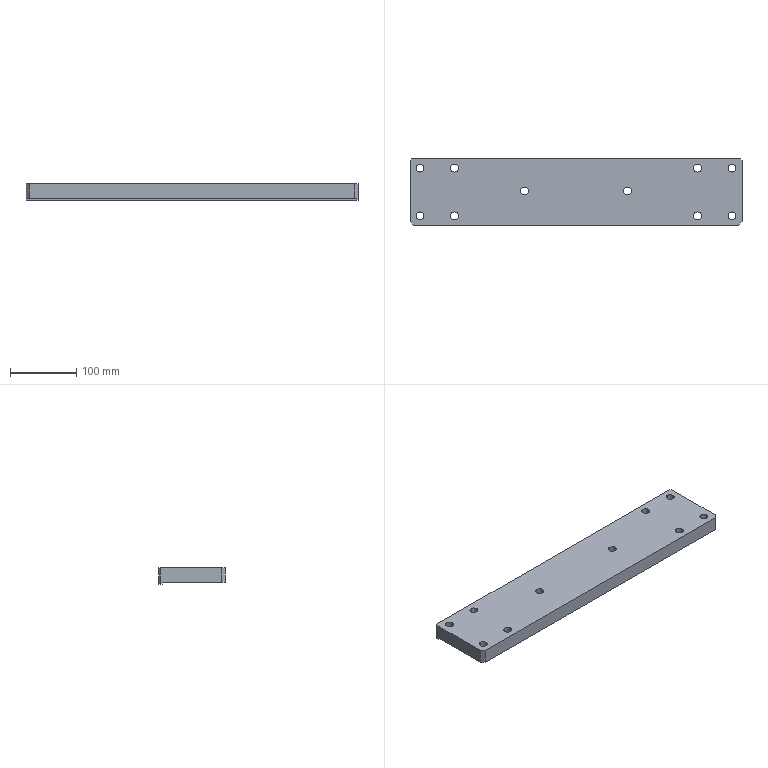Part | STEP file | J452-EBZ05-03-04-Part-1 | 1 solid | 32 faces | box 500 x 100 x 25 mm | volume 1081969 mm3 | cylinder 20 | plane 12 | commonest cylinder face diameters 12 x20